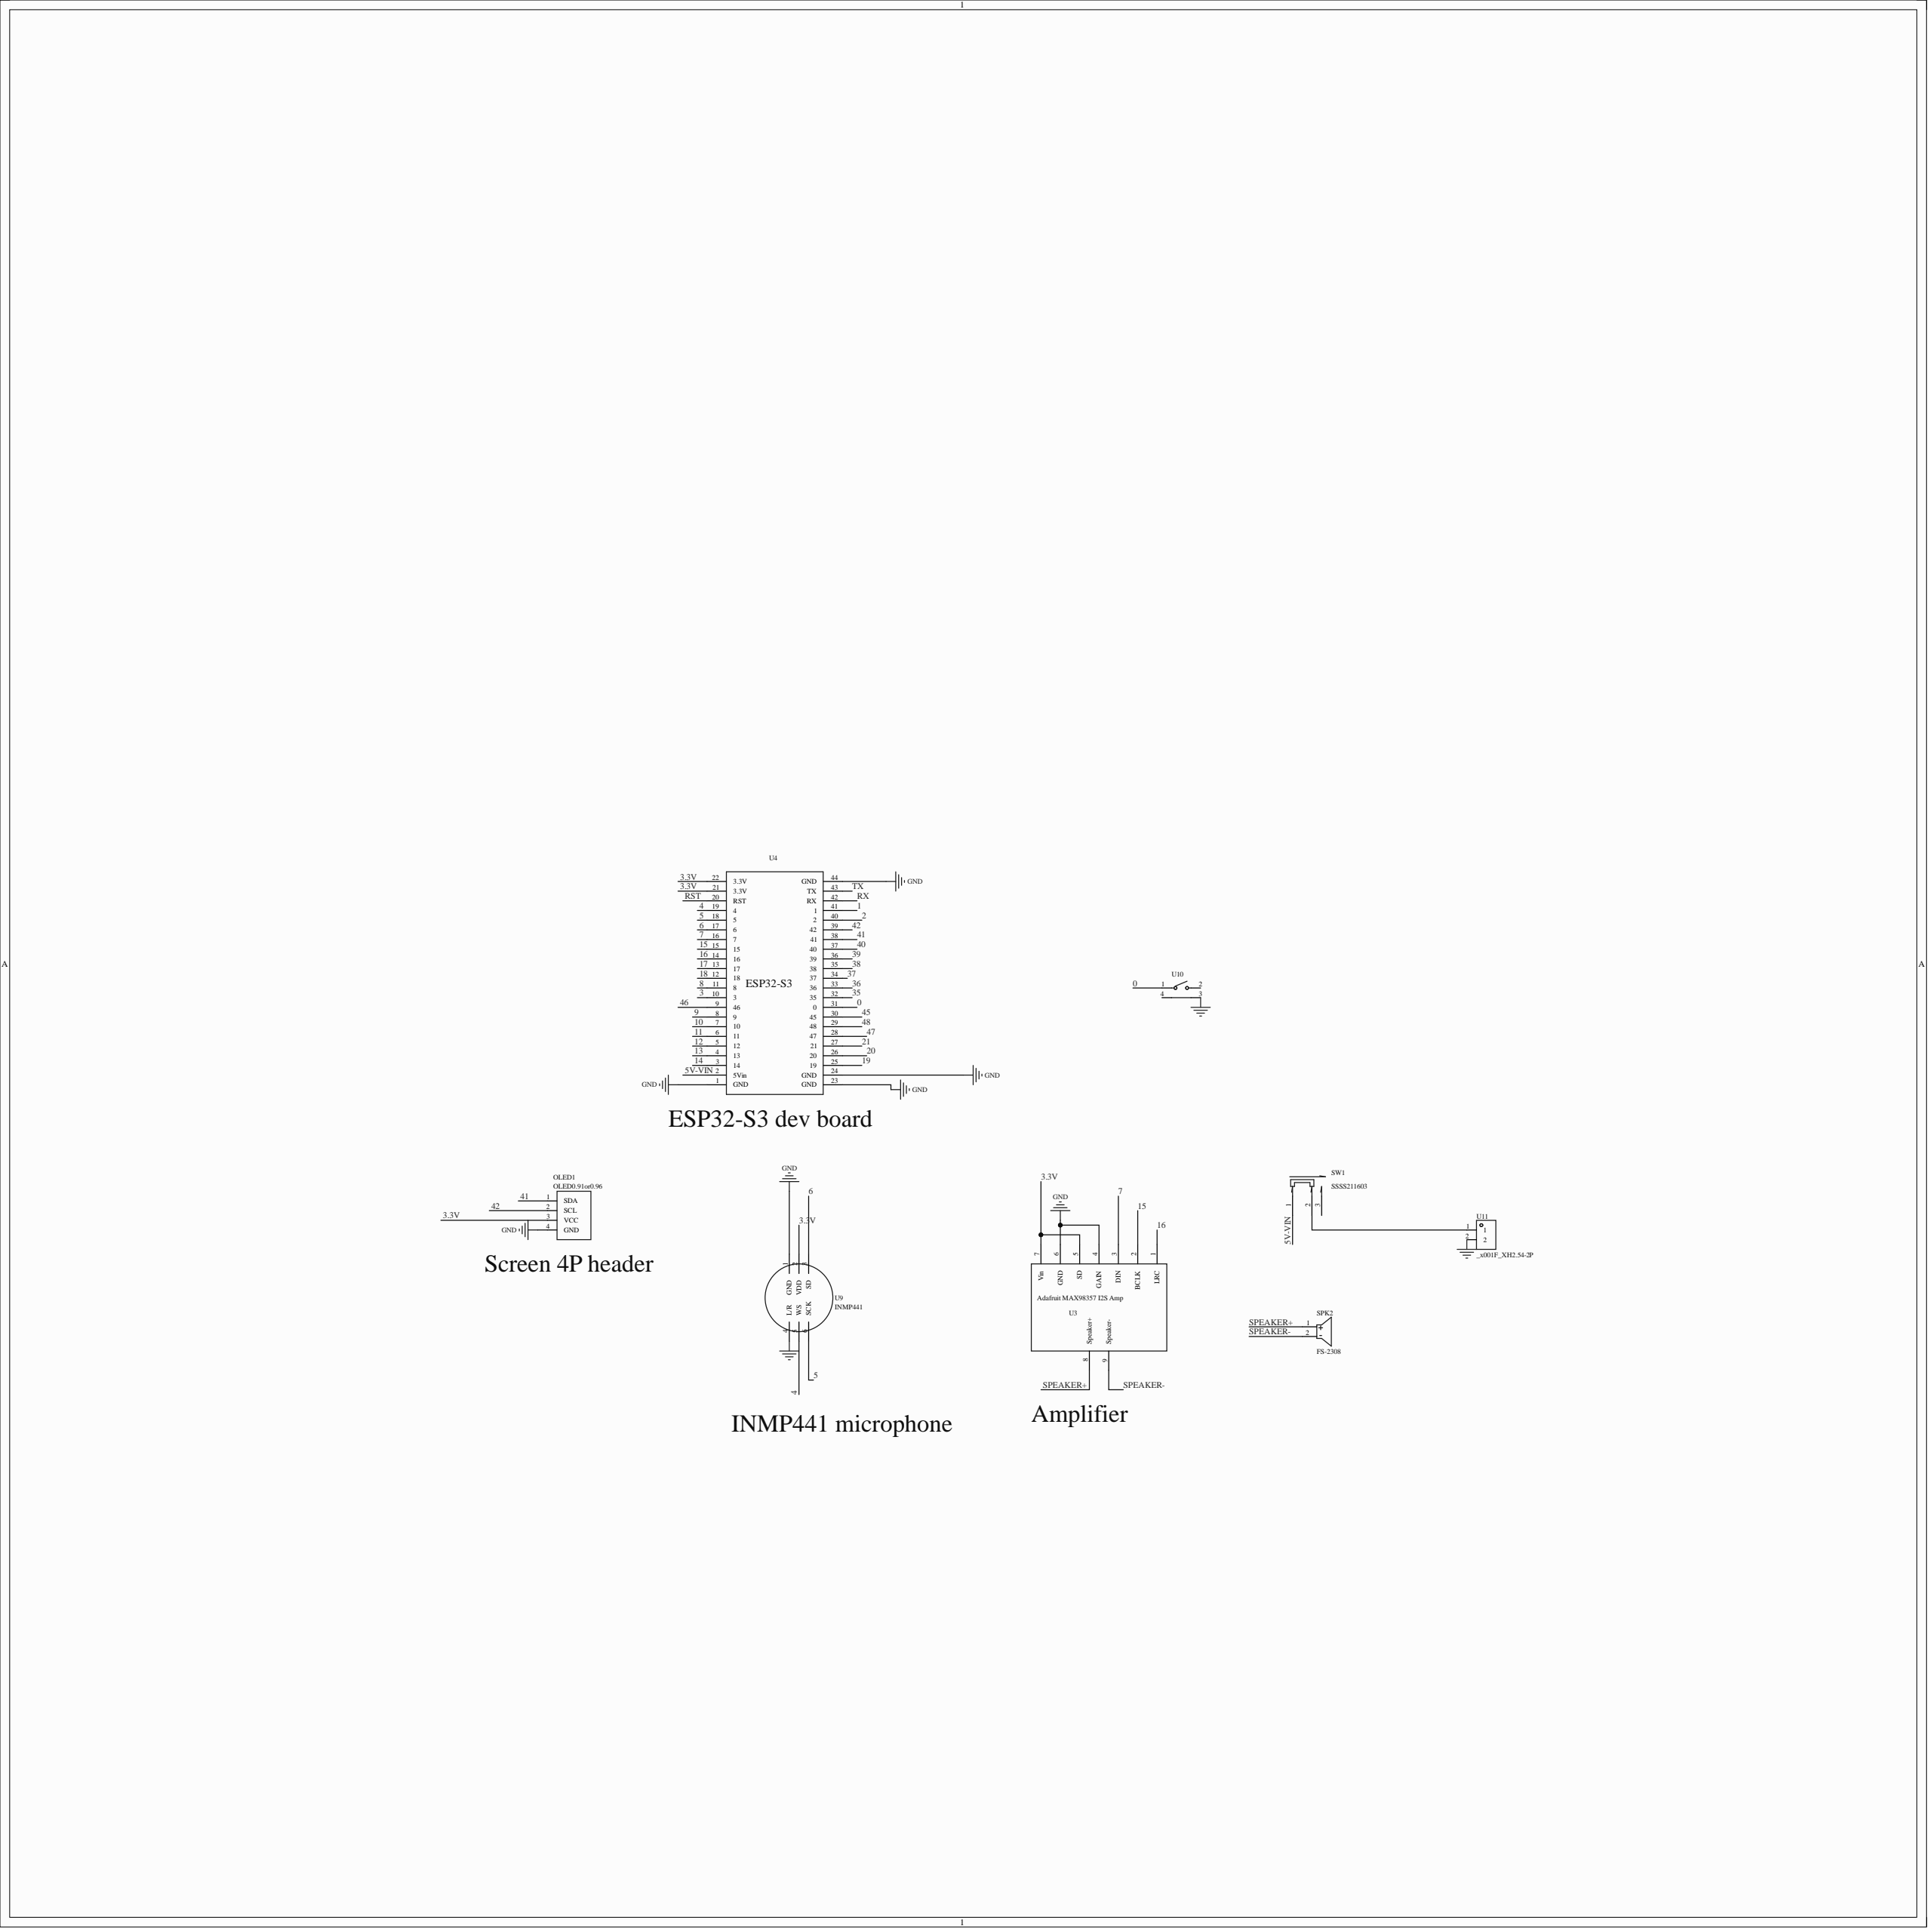Circuit board | Altium Designer | 8 parts | 15 nets
Bill of materials:
Comment,Description,Designator,Footprint,LibRef,Quantity
"OLED0.91or0.96","","OLED1","OLED0.91","OLED0.91or0.96","1"
"FS-2308","","SPK2","BEEP-TH_BD23.2-P9.20-D1.0","FS-2308","1"
"SSSS211603","","SW1","SW-SMD_SSSS211603","SSSS211603","1"
"Adafruit MAX98357 I2S Amp","","U3","MAX98357 I2S AMP MODULE","Adafruit MAX98357 I2S Amp","1"
"NO","","U4","ESP32S3","NO","1"
"INMP441","","U9","INMP441","INMP441","1"
"GT-TC054A-H038-L1","","U10","SW-SMD_L7.8-W3.5-P4.20-EH","GT-TC054A-H038-L1","1"
"_x001F_XH2.54-2P","","U11","CONN-TH_2P-P2.54-V","_x001F_XH2.54-2P","1"
Netlist (Protel format):
[
OLED1
OLED0.91
OLED0.91or0.96



]
[
SPK2
BEEP-TH_BD23.2-P9.20-D1.0
FS-2308



]
[
SW1
SW-SMD_SSSS211603
SSSS211603



]
[
U3
MAX98357 I2S AMP MODULE
Adafruit MAX98357 I2S Amp



]
[
U4
ESP32S3
NO



]
[
U9
INMP441
INMP441



]
[
U10
SW-SMD_L7.8-W3.5-P4.20-EH
GT-TC054A-H038-L1



]
[
U11
CONN-TH_2P-P2.54-V
_x001F_XH2.54-2P



]
(
SPEAKER-
SPK2-2
U3-9
)
(
SPEAKER+
SPK2-1
U3-8
)
(
NetSW1_2
SW1-2
U11-1
)
(
GND
OLED1-4
U3-4
U3-6
U4-1
U4-23
U4-24
U4-44
U9-1
U9-4
U10-3
U11-2
)
(
42
OLED1-2
U4-39
)
(
41
OLED1-1
U4-38
)
(
16
U3-1
U4-14
)
(
15
U3-2
U4-15
)
(
7
U3-3
U4-16
)
(
6
U4-17
U9-3
)
(
5V-VIN
SW1-1
U4-2
)
(
5
U4-18
U9-6
)
(
4
U4-19
U9-5
)
(
3.3V
OLED1-3
U3-5
U3-7
U4-21
U4-22
U9-2
)
(
0
U4-31
U10-1
)